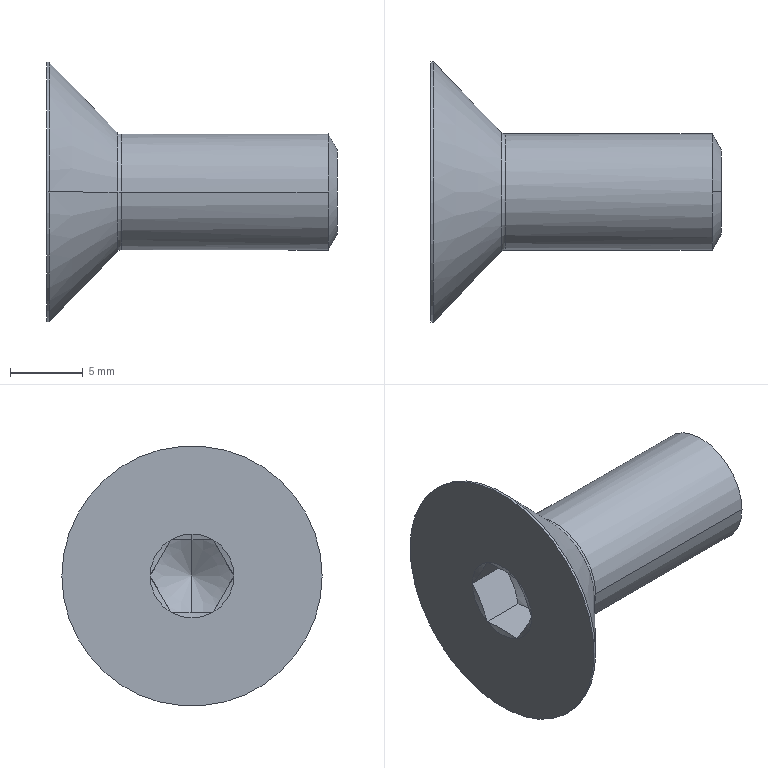Part | SolidWorks | features RevCut 2, Revolution 2, Cut 1, LPattern 1, RefAxis 1 | 1 solid | 27 faces | box 20 x 17.92 x 17.92 mm | volume 1375 mm3 | cone 13 | plane 8 | cylinder 4 | torus 2 | commonest cylinder face diameters 8 x2 17.92 x2
STEP:
#1=CARTESIAN_POINT('',(0.,0.,2.917));
#2=VERTEX_POINT('',#1);
#3=CARTESIAN_POINT('',(0.,0.,-2.917));
#4=VERTEX_POINT('',#3);
#5=CARTESIAN_POINT('',(0.,0.,0.));
#6=DIRECTION('',(-1.,0.,0.));
#7=DIRECTION('',(0.,0.,1.));
#8=AXIS2_PLACEMENT_3D('',#5,#6,#7);
#9=CIRCLE('',#8,2.917);
#10=EDGE_CURVE('',#2,#4,#9,.T.);
#11=ORIENTED_EDGE('',*,*,#10,.T.);
#12=CARTESIAN_POINT('',(-0.625,0.,-4.));
#13=VERTEX_POINT('',#12);
#14=CARTESIAN_POINT('',(-0.625,0.,-4.));
#15=DIRECTION('',(-0.5,0.,-0.866));
#16=VECTOR('',#15,1000.);
#17=LINE('',#14,#16);
#18=EDGE_CURVE('',#4,#13,#17,.T.);
#19=ORIENTED_EDGE('',*,*,#18,.T.);
#20=CARTESIAN_POINT('',(-0.625,4.,0.));
#21=VERTEX_POINT('',#20);
#22=CARTESIAN_POINT('',(-0.625,0.,0.));
#23=DIRECTION('',(-1.,0.,0.));
#24=DIRECTION('',(0.,0.,1.));
#25=AXIS2_PLACEMENT_3D('',#22,#23,#24);
#26=CIRCLE('',#25,4.);
#27=EDGE_CURVE('',#21,#13,#26,.T.);
#28=ORIENTED_EDGE('',*,*,#27,.F.);
#29=CARTESIAN_POINT('',(-0.625,0.,4.));
#30=VERTEX_POINT('',#29);
#31=CARTESIAN_POINT('',(-0.625,0.,0.));
#32=DIRECTION('',(-1.,0.,0.));
#33=DIRECTION('',(0.,0.,1.));
#34=AXIS2_PLACEMENT_3D('',#31,#32,#33);
#35=CIRCLE('',#34,4.);
#36=EDGE_CURVE('',#30,#21,#35,.T.);
#37=ORIENTED_EDGE('',*,*,#36,.F.);
#38=CARTESIAN_POINT('',(-0.625,0.,4.));
#39=DIRECTION('',(-0.5,0.,0.866));
#40=VECTOR('',#39,1000.);
#41=LINE('',#38,#40);
#42=EDGE_CURVE('',#2,#30,#41,.T.);
#43=ORIENTED_EDGE('',*,*,#42,.F.);
#44=EDGE_LOOP('',(#11,#19,#28,#37,#43));
#45=FACE_OUTER_BOUND('',#44,.T.);
#46=CARTESIAN_POINT('',(-0.625,0.,0.));
#47=DIRECTION('',(-1.,0.,0.));
#48=DIRECTION('',(0.,0.,1.));
#49=AXIS2_PLACEMENT_3D('',#46,#47,#48);
#50=CONICAL_SURFACE('',#49,4.,1.047);
#51=ADVANCED_FACE('',(#45),#50,.T.);
#52=CARTESIAN_POINT('',(-15.333,0.,0.));
#53=VERTEX_POINT('',#52);
#54=CARTESIAN_POINT('',(-16.777,0.,2.5));
#55=VERTEX_POINT('',#54);
#56=CARTESIAN_POINT('',(-17.,0.,2.887));
#57=DIRECTION('',(-0.5,0.,0.866));
#58=VECTOR('',#57,1000.);
#59=LINE('',#56,#58);
#60=EDGE_CURVE('',#53,#55,#59,.T.);
#61=ORIENTED_EDGE('',*,*,#60,.F.);
#62=CARTESIAN_POINT('',(-16.777,0.,-2.5));
#63=VERTEX_POINT('',#62);
#64=CARTESIAN_POINT('',(-17.,0.,-2.887));
#65=DIRECTION('',(-0.5,0.,-0.866));
#66=VECTOR('',#65,1000.);
#67=LINE('',#64,#66);
#68=EDGE_CURVE('',#53,#63,#67,.T.);
#69=ORIENTED_EDGE('',*,*,#68,.T.);
#70=CARTESIAN_POINT('',(-17.,-1.443,-2.5));
#71=VERTEX_POINT('',#70);
#72=CARTESIAN_POINT('',(-16.777,0.,-2.5));
#73=CARTESIAN_POINT('',(-16.777,-0.2437,-2.5));
#74=CARTESIAN_POINT('',(-16.798,-0.486,-2.5));
#75=CARTESIAN_POINT('',(-16.875,-0.9685,-2.5));
#76=CARTESIAN_POINT('',(-16.932,-1.209,-2.5));
#77=CARTESIAN_POINT('',(-17.,-1.443,-2.5));
#78=B_SPLINE_CURVE_WITH_KNOTS('',3,(#72,#73,#74,#75,#76,#77),.UNSPECIFIED.,.F.,.F.,(4,2,4),(0.009193,0.009923,0.01065),.UNSPECIFIED.);
#79=EDGE_CURVE('',#63,#71,#78,.T.);
#80=ORIENTED_EDGE('',*,*,#79,.T.);
#81=CARTESIAN_POINT('',(-17.,-2.887,0.));
#82=VERTEX_POINT('',#81);
#83=CARTESIAN_POINT('',(-17.,-1.443,-2.5));
#84=CARTESIAN_POINT('',(-16.864,-1.679,-2.092));
#85=CARTESIAN_POINT('',(-16.777,-1.918,-1.677));
#86=CARTESIAN_POINT('',(-16.777,-2.286,-1.04));
#87=CARTESIAN_POINT('',(-16.798,-2.409,-0.8275));
#88=CARTESIAN_POINT('',(-16.876,-2.65,-0.4104));
#89=CARTESIAN_POINT('',(-16.932,-2.769,-0.2044));
#90=CARTESIAN_POINT('',(-17.,-2.887,0.));
#91=B_SPLINE_CURVE_WITH_KNOTS('',3,(#83,#84,#85,#86,#87,#88,#89,#90),.UNSPECIFIED.,.F.,.F.,(4,2,2,4),(0.000000238,0.001458,0.002187,0.002916),.UNSPECIFIED.);
#92=EDGE_CURVE('',#71,#82,#91,.T.);
#93=ORIENTED_EDGE('',*,*,#92,.T.);
#94=CARTESIAN_POINT('',(-17.,-1.443,2.5));
#95=VERTEX_POINT('',#94);
#96=CARTESIAN_POINT('',(-17.,-2.887,0.));
#97=CARTESIAN_POINT('',(-16.864,-2.651,0.4082));
#98=CARTESIAN_POINT('',(-16.777,-2.412,0.8225));
#99=CARTESIAN_POINT('',(-16.777,-2.044,1.46));
#100=CARTESIAN_POINT('',(-16.798,-1.921,1.672));
#101=CARTESIAN_POINT('',(-16.876,-1.68,2.09));
#102=CARTESIAN_POINT('',(-16.932,-1.561,2.296));
#103=CARTESIAN_POINT('',(-17.,-1.443,2.5));
#104=B_SPLINE_CURVE_WITH_KNOTS('',3,(#96,#97,#98,#99,#100,#101,#102,#103),.UNSPECIFIED.,.F.,.F.,(4,2,2,4),(0.000000238,0.001458,0.002187,0.002916),.UNSPECIFIED.);
#105=EDGE_CURVE('',#82,#95,#104,.T.);
#106=ORIENTED_EDGE('',*,*,#105,.T.);
#107=CARTESIAN_POINT('',(-17.,-1.443,2.5));
#108=CARTESIAN_POINT('',(-16.932,-1.209,2.5));
#109=CARTESIAN_POINT('',(-16.875,-0.9685,2.5));
#110=CARTESIAN_POINT('',(-16.798,-0.486,2.5));
#111=CARTESIAN_POINT('',(-16.777,-0.2437,2.5));
#112=CARTESIAN_POINT('',(-16.777,0.,2.5));
#113=B_SPLINE_CURVE_WITH_KNOTS('',3,(#107,#108,#109,#110,#111,#112),.UNSPECIFIED.,.F.,.F.,(4,2,4),(0.002475,0.003205,0.003934),.UNSPECIFIED.);
#114=EDGE_CURVE('',#95,#55,#113,.T.);
#115=ORIENTED_EDGE('',*,*,#114,.T.);
#116=EDGE_LOOP('',(#61,#69,#80,#93,#106,#115));
#117=FACE_OUTER_BOUND('',#116,.T.);
#118=CARTESIAN_POINT('',(-17.,0.,0.));
#119=DIRECTION('',(-1.,0.,0.));
#120=DIRECTION('',(0.,0.,1.));
#121=AXIS2_PLACEMENT_3D('',#118,#119,#120);
#122=CONICAL_SURFACE('',#121,2.887,1.047);
#123=ADVANCED_FACE('',(#117),#122,.F.);
#124=CARTESIAN_POINT('',(-20.,1.443,2.5));
#125=VERTEX_POINT('',#124);
#126=CARTESIAN_POINT('',(-19.894,0.,2.5));
#127=VERTEX_POINT('',#126);
#128=CARTESIAN_POINT('',(-20.,1.443,2.5));
#129=CARTESIAN_POINT('',(-19.934,0.9633,2.5));
#130=CARTESIAN_POINT('',(-19.894,0.4823,2.5));
#131=CARTESIAN_POINT('',(-19.894,0.,2.5));
#132=B_SPLINE_CURVE_WITH_KNOTS('',3,(#128,#129,#130,#131),.UNSPECIFIED.,.F.,.F.,(4,4),(0.006027,0.00748),.UNSPECIFIED.);
#133=EDGE_CURVE('',#125,#127,#132,.T.);
#134=ORIENTED_EDGE('',*,*,#133,.T.);
#135=CARTESIAN_POINT('',(-20.,0.,2.887));
#136=VERTEX_POINT('',#135);
#137=CARTESIAN_POINT('',(-19.208,0.,0.));
#138=DIRECTION('',(-0.2646,0.,0.9644));
#139=VECTOR('',#138,1000.);
#140=LINE('',#137,#139);
#141=EDGE_CURVE('',#127,#136,#140,.T.);
#142=ORIENTED_EDGE('',*,*,#141,.T.);
#143=CARTESIAN_POINT('',(-20.,0.,0.));
#144=DIRECTION('',(1.,0.,0.));
#145=DIRECTION('',(0.,-1.,0.));
#146=AXIS2_PLACEMENT_3D('',#143,#144,#145);
#147=CIRCLE('',#146,2.887);
#148=EDGE_CURVE('',#125,#136,#147,.T.);
#149=ORIENTED_EDGE('',*,*,#148,.F.);
#150=EDGE_LOOP('',(#134,#142,#149));
#151=FACE_OUTER_BOUND('',#150,.T.);
#152=CARTESIAN_POINT('',(-1019.208,0.,0.));
#153=DIRECTION('',(-1.,0.,0.));
#154=DIRECTION('',(0.,0.,1.));
#155=AXIS2_PLACEMENT_3D('',#152,#153,#154);
#156=CONICAL_SURFACE('',#155,3644.888,1.303);
#157=ADVANCED_FACE('',(#151),#156,.F.);
#158=CARTESIAN_POINT('',(-14.87,-4.,0.));
#159=VERTEX_POINT('',#158);
#160=CARTESIAN_POINT('',(-14.87,4.,0.));
#161=VERTEX_POINT('',#160);
#162=CARTESIAN_POINT('',(-14.87,0.,0.));
#163=DIRECTION('',(1.,0.,0.));
#164=DIRECTION('',(0.,1.,0.));
#165=AXIS2_PLACEMENT_3D('',#162,#163,#164);
#166=CIRCLE('',#165,4.);
#167=EDGE_CURVE('',#159,#161,#166,.T.);
#168=ORIENTED_EDGE('',*,*,#167,.F.);
#169=CARTESIAN_POINT('',(-15.158,-4.122,0.));
#170=VERTEX_POINT('',#169);
#171=CARTESIAN_POINT('',(-14.87,-4.4,0.));
#172=DIRECTION('',(0.,0.,1.));
#173=DIRECTION('',(0.,-1.,0.));
#174=AXIS2_PLACEMENT_3D('',#171,#172,#173);
#175=CIRCLE('',#174,0.4);
#176=EDGE_CURVE('',#159,#170,#175,.T.);
#177=ORIENTED_EDGE('',*,*,#176,.T.);
#178=CARTESIAN_POINT('',(-15.158,4.122,0.));
#179=VERTEX_POINT('',#178);
#180=CARTESIAN_POINT('',(-15.158,0.,0.));
#181=DIRECTION('',(1.,0.,0.));
#182=DIRECTION('',(0.,1.,0.));
#183=AXIS2_PLACEMENT_3D('',#180,#181,#182);
#184=CIRCLE('',#183,4.122);
#185=EDGE_CURVE('',#170,#179,#184,.T.);
#186=ORIENTED_EDGE('',*,*,#185,.T.);
#187=CARTESIAN_POINT('',(-14.87,4.4,0.));
#188=DIRECTION('',(0.,0.,-1.));
#189=DIRECTION('',(-1.,0.,0.));
#190=AXIS2_PLACEMENT_3D('',#187,#188,#189);
#191=CIRCLE('',#190,0.4);
#192=EDGE_CURVE('',#161,#179,#191,.T.);
#193=ORIENTED_EDGE('',*,*,#192,.F.);
#194=EDGE_LOOP('',(#168,#177,#186,#193));
#195=FACE_OUTER_BOUND('',#194,.T.);
#196=CARTESIAN_POINT('',(-14.87,0.,0.));
#197=DIRECTION('',(1.,0.,0.));
#198=DIRECTION('',(0.,1.,0.));
#199=AXIS2_PLACEMENT_3D('',#196,#197,#198);
#200=TOROIDAL_SURFACE('',#199,4.4,0.4);
#201=ADVANCED_FACE('',(#195),#200,.F.);
#202=CARTESIAN_POINT('',(-15.158,0.,0.));
#203=DIRECTION('',(1.,0.,0.));
#204=DIRECTION('',(0.,1.,0.));
#205=AXIS2_PLACEMENT_3D('',#202,#203,#204);
#206=CIRCLE('',#205,4.122);
#207=EDGE_CURVE('',#179,#170,#206,.T.);
#208=ORIENTED_EDGE('',*,*,#207,.F.);
#209=CARTESIAN_POINT('',(-19.83,8.96,0.));
#210=VERTEX_POINT('',#209);
#211=CARTESIAN_POINT('',(-15.158,4.122,0.));
#212=DIRECTION('',(-0.6947,0.7193,0.));
#213=VECTOR('',#212,1000.);
#214=LINE('',#211,#213);
#215=EDGE_CURVE('',#179,#210,#214,.T.);
#216=ORIENTED_EDGE('',*,*,#215,.T.);
#217=CARTESIAN_POINT('',(-19.83,-8.96,0.));
#218=VERTEX_POINT('',#217);
#219=CARTESIAN_POINT('',(-19.83,0.,0.));
#220=DIRECTION('',(1.,0.,0.));
#221=DIRECTION('',(0.,1.,0.));
#222=AXIS2_PLACEMENT_3D('',#219,#220,#221);
#223=CIRCLE('',#222,8.96);
#224=EDGE_CURVE('',#210,#218,#223,.T.);
#225=ORIENTED_EDGE('',*,*,#224,.T.);
#226=CARTESIAN_POINT('',(-15.158,-4.122,0.));
#227=DIRECTION('',(-0.6947,-0.7193,0.));
#228=VECTOR('',#227,1000.);
#229=LINE('',#226,#228);
#230=EDGE_CURVE('',#170,#218,#229,.T.);
#231=ORIENTED_EDGE('',*,*,#230,.F.);
#232=EDGE_LOOP('',(#208,#216,#225,#231));
#233=FACE_OUTER_BOUND('',#232,.T.);
#234=CARTESIAN_POINT('',(-15.158,0.,0.));
#235=DIRECTION('',(-1.,0.,0.));
#236=DIRECTION('',(0.,-1.,0.));
#237=AXIS2_PLACEMENT_3D('',#234,#235,#236);
#238=CONICAL_SURFACE('',#237,4.122,0.8029);
#239=ADVANCED_FACE('',(#233),#238,.T.);
#240=CARTESIAN_POINT('',(-20.,8.96,0.));
#241=VERTEX_POINT('',#240);
#242=CARTESIAN_POINT('',(-20.,-8.96,0.));
#243=VERTEX_POINT('',#242);
#244=CARTESIAN_POINT('',(-20.,0.,0.));
#245=DIRECTION('',(1.,0.,0.));
#246=DIRECTION('',(0.,1.,0.));
#247=AXIS2_PLACEMENT_3D('',#244,#245,#246);
#248=CIRCLE('',#247,8.96);
#249=EDGE_CURVE('',#241,#243,#248,.T.);
#250=ORIENTED_EDGE('',*,*,#249,.T.);
#251=CARTESIAN_POINT('',(0.,-8.96,0.));
#252=DIRECTION('',(1.,0.,0.));
#253=VECTOR('',#252,1000.);
#254=LINE('',#251,#253);
#255=EDGE_CURVE('',#243,#218,#254,.T.);
#256=ORIENTED_EDGE('',*,*,#255,.T.);
#257=ORIENTED_EDGE('',*,*,#224,.F.);
#258=CARTESIAN_POINT('',(0.,8.96,0.));
#259=DIRECTION('',(1.,0.,0.));
#260=VECTOR('',#259,1000.);
#261=LINE('',#258,#260);
#262=EDGE_CURVE('',#241,#210,#261,.T.);
#263=ORIENTED_EDGE('',*,*,#262,.F.);
#264=EDGE_LOOP('',(#250,#256,#257,#263));
#265=FACE_OUTER_BOUND('',#264,.T.);
#266=CARTESIAN_POINT('',(0.,0.,0.));
#267=DIRECTION('',(1.,0.,0.));
#268=DIRECTION('',(0.,1.,0.));
#269=AXIS2_PLACEMENT_3D('',#266,#267,#268);
#270=CYLINDRICAL_SURFACE('',#269,8.96);
#271=ADVANCED_FACE('',(#265),#270,.T.);
#272=CARTESIAN_POINT('',(-14.87,0.,0.));
#273=DIRECTION('',(1.,0.,0.));
#274=DIRECTION('',(0.,1.,0.));
#275=AXIS2_PLACEMENT_3D('',#272,#273,#274);
#276=CIRCLE('',#275,4.);
#277=EDGE_CURVE('',#161,#159,#276,.T.);
#278=ORIENTED_EDGE('',*,*,#277,.T.);
#279=CARTESIAN_POINT('',(-0.625,-4.,0.));
#280=VERTEX_POINT('',#279);
#281=CARTESIAN_POINT('',(0.,-4.,0.));
#282=DIRECTION('',(1.,0.,0.));
#283=VECTOR('',#282,1000.);
#284=LINE('',#281,#283);
#285=EDGE_CURVE('',#159,#280,#284,.T.);
#286=ORIENTED_EDGE('',*,*,#285,.T.);
#287=CARTESIAN_POINT('',(-0.625,0.,0.));
#288=DIRECTION('',(-1.,0.,0.));
#289=DIRECTION('',(0.,0.,1.));
#290=AXIS2_PLACEMENT_3D('',#287,#288,#289);
#291=CIRCLE('',#290,4.);
#292=EDGE_CURVE('',#280,#30,#291,.T.);
#293=ORIENTED_EDGE('',*,*,#292,.T.);
#294=ORIENTED_EDGE('',*,*,#36,.T.);
#295=CARTESIAN_POINT('',(0.,4.,0.));
#296=DIRECTION('',(1.,0.,0.));
#297=VECTOR('',#296,1000.);
#298=LINE('',#295,#297);
#299=EDGE_CURVE('',#161,#21,#298,.T.);
#300=ORIENTED_EDGE('',*,*,#299,.F.);
#301=EDGE_LOOP('',(#278,#286,#293,#294,#300));
#302=FACE_OUTER_BOUND('',#301,.T.);
#303=CARTESIAN_POINT('',(0.,0.,0.));
#304=DIRECTION('',(1.,0.,0.));
#305=DIRECTION('',(0.,1.,0.));
#306=AXIS2_PLACEMENT_3D('',#303,#304,#305);
#307=CYLINDRICAL_SURFACE('',#306,4.);
#308=ADVANCED_FACE('',(#302),#307,.T.);
#309=ORIENTED_EDGE('',*,*,#285,.F.);
#310=ORIENTED_EDGE('',*,*,#167,.T.);
#311=ORIENTED_EDGE('',*,*,#299,.T.);
#312=ORIENTED_EDGE('',*,*,#27,.T.);
#313=CARTESIAN_POINT('',(-0.625,0.,0.));
#314=DIRECTION('',(-1.,0.,0.));
#315=DIRECTION('',(0.,0.,1.));
#316=AXIS2_PLACEMENT_3D('',#313,#314,#315);
#317=CIRCLE('',#316,4.);
#318=EDGE_CURVE('',#13,#280,#317,.T.);
#319=ORIENTED_EDGE('',*,*,#318,.T.);
#320=EDGE_LOOP('',(#309,#310,#311,#312,#319));
#321=FACE_OUTER_BOUND('',#320,.T.);
#322=CARTESIAN_POINT('',(0.,0.,0.));
#323=DIRECTION('',(1.,0.,0.));
#324=DIRECTION('',(0.,1.,0.));
#325=AXIS2_PLACEMENT_3D('',#322,#323,#324);
#326=CYLINDRICAL_SURFACE('',#325,4.);
#327=ADVANCED_FACE('',(#321),#326,.T.);
#328=ORIENTED_EDGE('',*,*,#249,.F.);
#329=CARTESIAN_POINT('',(-20.,0.,0.));
#330=DIRECTION('',(1.,0.,0.));
#331=DIRECTION('',(0.,1.,0.));
#332=AXIS2_PLACEMENT_3D('',#329,#330,#331);
#333=CIRCLE('',#332,8.96);
#334=EDGE_CURVE('',#243,#241,#333,.T.);
#335=ORIENTED_EDGE('',*,*,#334,.F.);
#336=EDGE_LOOP('',(#328,#335));
#337=FACE_OUTER_BOUND('',#336,.T.);
#338=CARTESIAN_POINT('',(-20.,-1.443,2.5));
#339=VERTEX_POINT('',#338);
#340=CARTESIAN_POINT('',(-20.,-2.887,0.));
#341=VERTEX_POINT('',#340);
#342=CARTESIAN_POINT('',(-20.,0.,0.));
#343=DIRECTION('',(1.,0.,0.));
#344=DIRECTION('',(0.,-1.,0.));
#345=AXIS2_PLACEMENT_3D('',#342,#343,#344);
#346=CIRCLE('',#345,2.887);
#347=EDGE_CURVE('',#339,#341,#346,.T.);
#348=ORIENTED_EDGE('',*,*,#347,.T.);
#349=CARTESIAN_POINT('',(-20.,-1.443,-2.5));
#350=VERTEX_POINT('',#349);
#351=CARTESIAN_POINT('',(-20.,0.,0.));
#352=DIRECTION('',(1.,0.,0.));
#353=DIRECTION('',(0.,-1.,0.));
#354=AXIS2_PLACEMENT_3D('',#351,#352,#353);
#355=CIRCLE('',#354,2.887);
#356=EDGE_CURVE('',#341,#350,#355,.T.);
#357=ORIENTED_EDGE('',*,*,#356,.T.);
#358=CARTESIAN_POINT('',(-20.,1.443,-2.5));
#359=VERTEX_POINT('',#358);
#360=CARTESIAN_POINT('',(-20.,0.,0.));
#361=DIRECTION('',(1.,0.,0.));
#362=DIRECTION('',(0.,-1.,0.));
#363=AXIS2_PLACEMENT_3D('',#360,#361,#362);
#364=CIRCLE('',#363,2.887);
#365=EDGE_CURVE('',#350,#359,#364,.T.);
#366=ORIENTED_EDGE('',*,*,#365,.T.);
#367=CARTESIAN_POINT('',(-20.,2.887,0.));
#368=VERTEX_POINT('',#367);
#369=CARTESIAN_POINT('',(-20.,0.,0.));
#370=DIRECTION('',(1.,0.,0.));
#371=DIRECTION('',(0.,-1.,0.));
#372=AXIS2_PLACEMENT_3D('',#369,#370,#371);
#373=CIRCLE('',#372,2.887);
#374=EDGE_CURVE('',#359,#368,#373,.T.);
#375=ORIENTED_EDGE('',*,*,#374,.T.);
#376=CARTESIAN_POINT('',(-20.,0.,0.));
#377=DIRECTION('',(-1.,0.,0.));
#378=DIRECTION('',(0.,0.,1.));
#379=AXIS2_PLACEMENT_3D('',#376,#377,#378);
#380=CIRCLE('',#379,2.887);
#381=EDGE_CURVE('',#125,#368,#380,.T.);
#382=ORIENTED_EDGE('',*,*,#381,.F.);
#383=ORIENTED_EDGE('',*,*,#148,.T.);
#384=CARTESIAN_POINT('',(-20.,0.,0.));
#385=DIRECTION('',(1.,0.,0.));
#386=DIRECTION('',(0.,-1.,0.));
#387=AXIS2_PLACEMENT_3D('',#384,#385,#386);
#388=CIRCLE('',#387,2.887);
#389=EDGE_CURVE('',#136,#339,#388,.T.);
#390=ORIENTED_EDGE('',*,*,#389,.T.);
#391=EDGE_LOOP('',(#348,#357,#366,#375,#382,#383,#390));
#392=FACE_BOUND('',#391,.T.);
#393=CARTESIAN_POINT('',(-20.,8.96,0.));
#394=DIRECTION('',(-1.,0.,0.));
#395=DIRECTION('',(0.,-1.,0.));
#396=AXIS2_PLACEMENT_3D('',#393,#394,#395);
#397=PLANE('',#396);
#398=ADVANCED_FACE('',(#337,#392),#397,.T.);
#399=ORIENTED_EDGE('',*,*,#255,.F.);
#400=ORIENTED_EDGE('',*,*,#334,.T.);
#401=ORIENTED_EDGE('',*,*,#262,.T.);
#402=CARTESIAN_POINT('',(-19.83,0.,0.));
#403=DIRECTION('',(1.,0.,0.));
#404=DIRECTION('',(0.,1.,0.));
#405=AXIS2_PLACEMENT_3D('',#402,#403,#404);
#406=CIRCLE('',#405,8.96);
#407=EDGE_CURVE('',#218,#210,#406,.T.);
#408=ORIENTED_EDGE('',*,*,#407,.F.);
#409=EDGE_LOOP('',(#399,#400,#401,#408));
#410=FACE_OUTER_BOUND('',#409,.T.);
#411=CARTESIAN_POINT('',(0.,0.,0.));
#412=DIRECTION('',(1.,0.,0.));
#413=DIRECTION('',(0.,1.,0.));
#414=AXIS2_PLACEMENT_3D('',#411,#412,#413);
#415=CYLINDRICAL_SURFACE('',#414,8.96);
#416=ADVANCED_FACE('',(#410),#415,.T.);
#417=ORIENTED_EDGE('',*,*,#215,.F.);
#418=ORIENTED_EDGE('',*,*,#185,.F.);
#419=ORIENTED_EDGE('',*,*,#230,.T.);
#420=ORIENTED_EDGE('',*,*,#407,.T.);
#421=EDGE_LOOP('',(#417,#418,#419,#420));
#422=FACE_OUTER_BOUND('',#421,.T.);
#423=CARTESIAN_POINT('',(-15.158,0.,0.));
#424=DIRECTION('',(-1.,0.,0.));
#425=DIRECTION('',(0.,-1.,0.));
#426=AXIS2_PLACEMENT_3D('',#423,#424,#425);
#427=CONICAL_SURFACE('',#426,4.122,0.8029);
#428=ADVANCED_FACE('',(#422),#427,.T.);
#429=ORIENTED_EDGE('',*,*,#176,.F.);
#430=ORIENTED_EDGE('',*,*,#277,.F.);
#431=ORIENTED_EDGE('',*,*,#192,.T.);
#432=ORIENTED_EDGE('',*,*,#207,.T.);
#433=EDGE_LOOP('',(#429,#430,#431,#432));
#434=FACE_OUTER_BOUND('',#433,.T.);
#435=CARTESIAN_POINT('',(-14.87,0.,0.));
#436=DIRECTION('',(1.,0.,0.));
#437=DIRECTION('',(0.,1.,0.));
#438=AXIS2_PLACEMENT_3D('',#435,#436,#437);
#439=TOROIDAL_SURFACE('',#438,4.4,0.4);
#440=ADVANCED_FACE('',(#434),#439,.F.);
#441=CARTESIAN_POINT('',(-20.,-1.443,2.5));
#442=CARTESIAN_POINT('',(-19.934,-1.684,2.083));
#443=CARTESIAN_POINT('',(-19.854,-2.165,1.25));
#444=CARTESIAN_POINT('',(-19.934,-2.646,0.4167));
#445=CARTESIAN_POINT('',(-20.,-2.887,0.));
#446=B_SPLINE_CURVE_WITH_KNOTS('',3,(#441,#442,#443,#444,#445),.UNSPECIFIED.,.F.,.F.,(4,1,4),(0.000000231,0.001444,0.002887),.UNSPECIFIED.);
#447=EDGE_CURVE('',#339,#341,#446,.T.);
#448=ORIENTED_EDGE('',*,*,#447,.T.);
#449=ORIENTED_EDGE('',*,*,#347,.F.);
#450=EDGE_LOOP('',(#448,#449));
#451=FACE_OUTER_BOUND('',#450,.T.);
#452=CARTESIAN_POINT('',(-1019.208,0.,0.));
#453=DIRECTION('',(-1.,0.,0.));
#454=DIRECTION('',(0.,0.,1.));
#455=AXIS2_PLACEMENT_3D('',#452,#453,#454);
#456=CONICAL_SURFACE('',#455,3644.888,1.303);
#457=ADVANCED_FACE('',(#451),#456,.F.);
#458=ORIENTED_EDGE('',*,*,#141,.F.);
#459=CARTESIAN_POINT('',(-19.894,0.,2.5));
#460=CARTESIAN_POINT('',(-19.894,-0.4804,2.5));
#461=CARTESIAN_POINT('',(-19.934,-0.964,2.5));
#462=CARTESIAN_POINT('',(-20.,-1.443,2.5));
#463=B_SPLINE_CURVE_WITH_KNOTS('',3,(#459,#460,#461,#462),.UNSPECIFIED.,.F.,.F.,(4,4),(0.00748,0.008928),.UNSPECIFIED.);
#464=EDGE_CURVE('',#127,#339,#463,.T.);
#465=ORIENTED_EDGE('',*,*,#464,.T.);
#466=ORIENTED_EDGE('',*,*,#389,.F.);
#467=EDGE_LOOP('',(#458,#465,#466));
#468=FACE_OUTER_BOUND('',#467,.T.);
#469=CARTESIAN_POINT('',(-1019.208,0.,0.));
#470=DIRECTION('',(-1.,0.,0.));
#471=DIRECTION('',(0.,0.,1.));
#472=AXIS2_PLACEMENT_3D('',#469,#470,#471);
#473=CONICAL_SURFACE('',#472,3644.888,1.303);
#474=ADVANCED_FACE('',(#468),#473,.F.);
#475=CARTESIAN_POINT('',(-20.,2.887,0.));
#476=CARTESIAN_POINT('',(-19.934,2.646,0.4167));
#477=CARTESIAN_POINT('',(-19.854,2.165,1.25));
#478=CARTESIAN_POINT('',(-19.934,1.684,2.083));
#479=CARTESIAN_POINT('',(-20.,1.443,2.5));
#480=B_SPLINE_CURVE_WITH_KNOTS('',3,(#475,#476,#477,#478,#479),.UNSPECIFIED.,.F.,.F.,(4,1,4),(0.000000231,0.001444,0.002887),.UNSPECIFIED.);
#481=EDGE_CURVE('',#368,#125,#480,.T.);
#482=ORIENTED_EDGE('',*,*,#481,.T.);
#483=ORIENTED_EDGE('',*,*,#381,.T.);
#484=EDGE_LOOP('',(#482,#483));
#485=FACE_OUTER_BOUND('',#484,.T.);
#486=CARTESIAN_POINT('',(-1019.208,0.,0.));
#487=DIRECTION('',(-1.,0.,0.));
#488=DIRECTION('',(0.,0.,1.));
#489=AXIS2_PLACEMENT_3D('',#486,#487,#488);
#490=CONICAL_SURFACE('',#489,3644.888,1.303);
#491=ADVANCED_FACE('',(#485),#490,.F.);
#492=CARTESIAN_POINT('',(-20.,1.443,-2.5));
#493=CARTESIAN_POINT('',(-19.934,1.684,-2.083));
#494=CARTESIAN_POINT('',(-19.854,2.165,-1.25));
#495=CARTESIAN_POINT('',(-19.934,2.646,-0.4167));
#496=CARTESIAN_POINT('',(-20.,2.887,0.));
#497=B_SPLINE_CURVE_WITH_KNOTS('',3,(#492,#493,#494,#495,#496),.UNSPECIFIED.,.F.,.F.,(4,1,4),(0.000000231,0.001444,0.002887),.UNSPECIFIED.);
#498=EDGE_CURVE('',#359,#368,#497,.T.);
#499=ORIENTED_EDGE('',*,*,#498,.T.);
#500=ORIENTED_EDGE('',*,*,#374,.F.);
#501=EDGE_LOOP('',(#499,#500));
#502=FACE_OUTER_BOUND('',#501,.T.);
#503=CARTESIAN_POINT('',(-1019.208,0.,0.));
#504=DIRECTION('',(-1.,0.,0.));
#505=DIRECTION('',(0.,0.,1.));
#506=AXIS2_PLACEMENT_3D('',#503,#504,#505);
#507=CONICAL_SURFACE('',#506,3644.888,1.303);
#508=ADVANCED_FACE('',(#502),#507,.F.);
#509=CARTESIAN_POINT('',(-20.,-1.443,-2.5));
#510=CARTESIAN_POINT('',(-19.934,-0.963,-2.5));
#511=CARTESIAN_POINT('',(-19.894,-0.4785,-2.5));
#512=CARTESIAN_POINT('',(-19.894,0.4842,-2.5));
#513=CARTESIAN_POINT('',(-19.934,0.9642,-2.5));
#514=CARTESIAN_POINT('',(-20.,1.443,-2.5));
#515=B_SPLINE_CURVE_WITH_KNOTS('',3,(#509,#510,#511,#512,#513,#514),.UNSPECIFIED.,.F.,.F.,(4,2,4),(0.002365,0.003819,0.005272),.UNSPECIFIED.);
#516=EDGE_CURVE('',#350,#359,#515,.T.);
#517=ORIENTED_EDGE('',*,*,#516,.T.);
#518=ORIENTED_EDGE('',*,*,#365,.F.);
#519=EDGE_LOOP('',(#517,#518));
#520=FACE_OUTER_BOUND('',#519,.T.);
#521=CARTESIAN_POINT('',(-1019.208,0.,0.));
#522=DIRECTION('',(-1.,0.,0.));
#523=DIRECTION('',(0.,0.,1.));
#524=AXIS2_PLACEMENT_3D('',#521,#522,#523);
#525=CONICAL_SURFACE('',#524,3644.888,1.303);
#526=ADVANCED_FACE('',(#520),#525,.F.);
#527=CARTESIAN_POINT('',(-20.,-2.887,0.));
#528=CARTESIAN_POINT('',(-19.934,-2.646,-0.4167));
#529=CARTESIAN_POINT('',(-19.854,-2.165,-1.25));
#530=CARTESIAN_POINT('',(-19.934,-1.684,-2.083));
#531=CARTESIAN_POINT('',(-20.,-1.443,-2.5));
#532=B_SPLINE_CURVE_WITH_KNOTS('',3,(#527,#528,#529,#530,#531),.UNSPECIFIED.,.F.,.F.,(4,1,4),(0.000000231,0.001444,0.002887),.UNSPECIFIED.);
#533=EDGE_CURVE('',#341,#350,#532,.T.);
#534=ORIENTED_EDGE('',*,*,#533,.T.);
#535=ORIENTED_EDGE('',*,*,#356,.F.);
#536=EDGE_LOOP('',(#534,#535));
#537=FACE_OUTER_BOUND('',#536,.T.);
#538=CARTESIAN_POINT('',(-1019.208,0.,0.));
#539=DIRECTION('',(-1.,0.,0.));
#540=DIRECTION('',(0.,0.,1.));
#541=AXIS2_PLACEMENT_3D('',#538,#539,#540);
#542=CONICAL_SURFACE('',#541,3644.888,1.303);
#543=ADVANCED_FACE('',(#537),#542,.F.);
#544=ORIENTED_EDGE('',*,*,#68,.F.);
#545=ORIENTED_EDGE('',*,*,#60,.T.);
#546=CARTESIAN_POINT('',(-17.,1.443,2.5));
#547=VERTEX_POINT('',#546);
#548=CARTESIAN_POINT('',(-16.777,0.,2.5));
#549=CARTESIAN_POINT('',(-16.777,0.2438,2.5));
#550=CARTESIAN_POINT('',(-16.798,0.4909,2.5));
#551=CARTESIAN_POINT('',(-16.876,0.9735,2.5));
#552=CARTESIAN_POINT('',(-16.933,1.21,2.5));
#553=CARTESIAN_POINT('',(-17.,1.443,2.5));
#554=B_SPLINE_CURVE_WITH_KNOTS('',3,(#548,#549,#550,#551,#552,#553),.UNSPECIFIED.,.F.,.F.,(4,2,4),(0.003934,0.004664,0.005394),.UNSPECIFIED.);
#555=EDGE_CURVE('',#55,#547,#554,.T.);
#556=ORIENTED_EDGE('',*,*,#555,.T.);
#557=CARTESIAN_POINT('',(-17.,2.887,0.));
#558=VERTEX_POINT('',#557);
#559=CARTESIAN_POINT('',(-17.,1.443,2.5));
#560=CARTESIAN_POINT('',(-16.864,1.679,2.092));
#561=CARTESIAN_POINT('',(-16.777,1.918,1.677));
#562=CARTESIAN_POINT('',(-16.777,2.286,1.04));
#563=CARTESIAN_POINT('',(-16.798,2.409,0.8275));
#564=CARTESIAN_POINT('',(-16.876,2.65,0.4104));
#565=CARTESIAN_POINT('',(-16.932,2.769,0.2044));
#566=CARTESIAN_POINT('',(-17.,2.887,0.));
#567=B_SPLINE_CURVE_WITH_KNOTS('',3,(#559,#560,#561,#562,#563,#564,#565,#566),.UNSPECIFIED.,.F.,.F.,(4,2,2,4),(0.000000238,0.001458,0.002187,0.002916),.UNSPECIFIED.);
#568=EDGE_CURVE('',#547,#558,#567,.T.);
#569=ORIENTED_EDGE('',*,*,#568,.T.);
#570=CARTESIAN_POINT('',(-17.,1.443,-2.5));
#571=VERTEX_POINT('',#570);
#572=CARTESIAN_POINT('',(-17.,2.887,0.));
#573=CARTESIAN_POINT('',(-16.864,2.651,-0.4082));
#574=CARTESIAN_POINT('',(-16.777,2.412,-0.8225));
#575=CARTESIAN_POINT('',(-16.777,2.044,-1.46));
#576=CARTESIAN_POINT('',(-16.798,1.921,-1.672));
#577=CARTESIAN_POINT('',(-16.876,1.68,-2.09));
#578=CARTESIAN_POINT('',(-16.932,1.561,-2.296));
#579=CARTESIAN_POINT('',(-17.,1.443,-2.5));
#580=B_SPLINE_CURVE_WITH_KNOTS('',3,(#572,#573,#574,#575,#576,#577,#578,#579),.UNSPECIFIED.,.F.,.F.,(4,2,2,4),(0.000000238,0.001458,0.002187,0.002916),.UNSPECIFIED.);
#581=EDGE_CURVE('',#558,#571,#580,.T.);
#582=ORIENTED_EDGE('',*,*,#581,.T.);
#583=CARTESIAN_POINT('',(-17.,1.443,-2.5));
#584=CARTESIAN_POINT('',(-16.933,1.21,-2.5));
#585=CARTESIAN_POINT('',(-16.876,0.9735,-2.5));
#586=CARTESIAN_POINT('',(-16.798,0.4909,-2.5));
#587=CARTESIAN_POINT('',(-16.777,0.2438,-2.5));
#588=CARTESIAN_POINT('',(-16.777,0.,-2.5));
#589=B_SPLINE_CURVE_WITH_KNOTS('',3,(#583,#584,#585,#586,#587,#588),.UNSPECIFIED.,.F.,.F.,(4,2,4),(0.007731,0.008462,0.009193),.UNSPECIFIED.);
#590=EDGE_CURVE('',#571,#63,#589,.T.);
#591=ORIENTED_EDGE('',*,*,#590,.T.);
#592=EDGE_LOOP('',(#544,#545,#556,#569,#582,#591));
#593=FACE_OUTER_BOUND('',#592,.T.);
#594=CARTESIAN_POINT('',(-17.,0.,0.));
#595=DIRECTION('',(-1.,0.,0.));
#596=DIRECTION('',(0.,0.,1.));
#597=AXIS2_PLACEMENT_3D('',#594,#595,#596);
#598=CONICAL_SURFACE('',#597,2.887,1.047);
#599=ADVANCED_FACE('',(#593),#598,.F.);
#600=ORIENTED_EDGE('',*,*,#498,.F.);
#601=CARTESIAN_POINT('',(-14.94,1.443,-2.5));
#602=DIRECTION('',(-1.,0.,0.));
#603=VECTOR('',#602,1000.);
#604=LINE('',#601,#603);
#605=EDGE_CURVE('',#571,#359,#604,.T.);
#606=ORIENTED_EDGE('',*,*,#605,.F.);
#607=ORIENTED_EDGE('',*,*,#581,.F.);
#608=CARTESIAN_POINT('',(-14.94,2.887,0.));
#609=DIRECTION('',(-1.,0.,0.));
#610=VECTOR('',#609,1000.);
#611=LINE('',#608,#610);
#612=EDGE_CURVE('',#558,#368,#611,.T.);
#613=ORIENTED_EDGE('',*,*,#612,.T.);
#614=EDGE_LOOP('',(#600,#606,#607,#613));
#615=FACE_OUTER_BOUND('',#614,.T.);
#616=CARTESIAN_POINT('',(-14.94,2.887,0.));
#617=DIRECTION('',(0.,0.866,-0.5));
#618=DIRECTION('',(0.,0.5,0.866));
#619=AXIS2_PLACEMENT_3D('',#616,#617,#618);
#620=PLANE('',#619);
#621=ADVANCED_FACE('',(#615),#620,.F.);
#622=ORIENTED_EDGE('',*,*,#516,.F.);
#623=CARTESIAN_POINT('',(-14.94,-1.443,-2.5));
#624=DIRECTION('',(-1.,0.,0.));
#625=VECTOR('',#624,1000.);
#626=LINE('',#623,#625);
#627=EDGE_CURVE('',#71,#350,#626,.T.);
#628=ORIENTED_EDGE('',*,*,#627,.F.);
#629=ORIENTED_EDGE('',*,*,#79,.F.);
#630=ORIENTED_EDGE('',*,*,#590,.F.);
#631=ORIENTED_EDGE('',*,*,#605,.T.);
#632=EDGE_LOOP('',(#622,#628,#629,#630,#631));
#633=FACE_OUTER_BOUND('',#632,.T.);
#634=CARTESIAN_POINT('',(-14.94,1.443,-2.5));
#635=DIRECTION('',(0.,0.,-1.));
#636=DIRECTION('',(-1.,0.,0.));
#637=AXIS2_PLACEMENT_3D('',#634,#635,#636);
#638=PLANE('',#637);
#639=ADVANCED_FACE('',(#633),#638,.F.);
#640=ORIENTED_EDGE('',*,*,#533,.F.);
#641=CARTESIAN_POINT('',(-14.94,-2.887,0.));
#642=DIRECTION('',(-1.,0.,0.));
#643=VECTOR('',#642,1000.);
#644=LINE('',#641,#643);
#645=EDGE_CURVE('',#82,#341,#644,.T.);
#646=ORIENTED_EDGE('',*,*,#645,.F.);
#647=ORIENTED_EDGE('',*,*,#92,.F.);
#648=ORIENTED_EDGE('',*,*,#627,.T.);
#649=EDGE_LOOP('',(#640,#646,#647,#648));
#650=FACE_OUTER_BOUND('',#649,.T.);
#651=CARTESIAN_POINT('',(-14.94,-1.443,-2.5));
#652=DIRECTION('',(0.,-0.866,-0.5));
#653=DIRECTION('',(0.,0.5,-0.866));
#654=AXIS2_PLACEMENT_3D('',#651,#652,#653);
#655=PLANE('',#654);
#656=ADVANCED_FACE('',(#650),#655,.F.);
#657=ORIENTED_EDGE('',*,*,#447,.F.);
#658=CARTESIAN_POINT('',(-14.94,-1.443,2.5));
#659=DIRECTION('',(-1.,0.,0.));
#660=VECTOR('',#659,1000.);
#661=LINE('',#658,#660);
#662=EDGE_CURVE('',#95,#339,#661,.T.);
#663=ORIENTED_EDGE('',*,*,#662,.F.);
#664=ORIENTED_EDGE('',*,*,#105,.F.);
#665=ORIENTED_EDGE('',*,*,#645,.T.);
#666=EDGE_LOOP('',(#657,#663,#664,#665));
#667=FACE_OUTER_BOUND('',#666,.T.);
#668=CARTESIAN_POINT('',(-14.94,-2.887,0.));
#669=DIRECTION('',(0.,-0.866,0.5));
#670=DIRECTION('',(0.,-0.5,-0.866));
#671=AXIS2_PLACEMENT_3D('',#668,#669,#670);
#672=PLANE('',#671);
#673=ADVANCED_FACE('',(#667),#672,.F.);
#674=ORIENTED_EDGE('',*,*,#133,.F.);
#675=CARTESIAN_POINT('',(-14.94,1.443,2.5));
#676=DIRECTION('',(-1.,0.,0.));
#677=VECTOR('',#676,1000.);
#678=LINE('',#675,#677);
#679=EDGE_CURVE('',#547,#125,#678,.T.);
#680=ORIENTED_EDGE('',*,*,#679,.F.);
#681=ORIENTED_EDGE('',*,*,#555,.F.);
#682=ORIENTED_EDGE('',*,*,#114,.F.);
#683=ORIENTED_EDGE('',*,*,#662,.T.);
#684=ORIENTED_EDGE('',*,*,#464,.F.);
#685=EDGE_LOOP('',(#674,#680,#681,#682,#683,#684));
#686=FACE_OUTER_BOUND('',#685,.T.);
#687=CARTESIAN_POINT('',(-14.94,-1.443,2.5));
#688=DIRECTION('',(0.,0.,1.));
#689=DIRECTION('',(1.,0.,0.));
#690=AXIS2_PLACEMENT_3D('',#687,#688,#689);
#691=PLANE('',#690);
#692=ADVANCED_FACE('',(#686),#691,.F.);
#693=ORIENTED_EDGE('',*,*,#481,.F.);
#694=ORIENTED_EDGE('',*,*,#612,.F.);
#695=ORIENTED_EDGE('',*,*,#568,.F.);
#696=ORIENTED_EDGE('',*,*,#679,.T.);
#697=EDGE_LOOP('',(#693,#694,#695,#696));
#698=FACE_OUTER_BOUND('',#697,.T.);
#699=CARTESIAN_POINT('',(-14.94,1.443,2.5));
#700=DIRECTION('',(0.,0.866,0.5));
#701=DIRECTION('',(0.,-0.5,0.866));
#702=AXIS2_PLACEMENT_3D('',#699,#700,#701);
#703=PLANE('',#702);
#704=ADVANCED_FACE('',(#698),#703,.F.);
#705=ORIENTED_EDGE('',*,*,#18,.F.);
#706=CARTESIAN_POINT('',(0.,0.,0.));
#707=DIRECTION('',(-1.,0.,0.));
#708=DIRECTION('',(0.,0.,1.));
#709=AXIS2_PLACEMENT_3D('',#706,#707,#708);
#710=CIRCLE('',#709,2.917);
#711=EDGE_CURVE('',#4,#2,#710,.T.);
#712=ORIENTED_EDGE('',*,*,#711,.T.);
#713=ORIENTED_EDGE('',*,*,#42,.T.);
#714=ORIENTED_EDGE('',*,*,#292,.F.);
#715=ORIENTED_EDGE('',*,*,#318,.F.);
#716=EDGE_LOOP('',(#705,#712,#713,#714,#715));
#717=FACE_OUTER_BOUND('',#716,.T.);
#718=CARTESIAN_POINT('',(-0.625,0.,0.));
#719=DIRECTION('',(-1.,0.,0.));
#720=DIRECTION('',(0.,0.,1.));
#721=AXIS2_PLACEMENT_3D('',#718,#719,#720);
#722=CONICAL_SURFACE('',#721,4.,1.047);
#723=ADVANCED_FACE('',(#717),#722,.T.);
#724=ORIENTED_EDGE('',*,*,#10,.F.);
#725=ORIENTED_EDGE('',*,*,#711,.F.);
#726=EDGE_LOOP('',(#724,#725));
#727=FACE_OUTER_BOUND('',#726,.T.);
#728=CARTESIAN_POINT('',(0.,0.,0.));
#729=DIRECTION('',(1.,0.,0.));
#730=DIRECTION('',(0.,1.,0.));
#731=AXIS2_PLACEMENT_3D('',#728,#729,#730);
#732=PLANE('',#731);
#733=ADVANCED_FACE('',(#727),#732,.T.);
#734=CLOSED_SHELL('',(#51,#123,#157,#201,#239,#271,#308,#327,#398,#416,#428,#440,#457,#474,#491,#508,#526,#543,#599,#621,#639,#656,#673,#692,#704,#723,#733));
#735=MANIFOLD_SOLID_BREP('',#734);
#736=CARTESIAN_POINT('',(0.,0.,0.));
#737=DIRECTION('',(0.,0.,1.));
#738=DIRECTION('',(1.,0.,0.));
#739=AXIS2_PLACEMENT_3D('',#736,#737,#738);
#740=(LENGTH_UNIT()NAMED_UNIT(*)SI_UNIT(.MILLI.,.METRE.));
#741=UNCERTAINTY_MEASURE_WITH_UNIT(LENGTH_MEASURE(0.00001),#740,'','');
#742=(NAMED_UNIT(*)PLANE_ANGLE_UNIT()SI_UNIT($,.RADIAN.));
#743=(NAMED_UNIT(*)SI_UNIT($,.STERADIAN.)SOLID_ANGLE_UNIT());
#744=(GEOMETRIC_REPRESENTATION_CONTEXT(3)GLOBAL_UNCERTAINTY_ASSIGNED_CONTEXT((#741))GLOBAL_UNIT_ASSIGNED_CONTEXT((#740,#742,#743))REPRESENTATION_CONTEXT('',''));
#745=ADVANCED_BREP_SHAPE_REPRESENTATION('',(#735,#739),#744);